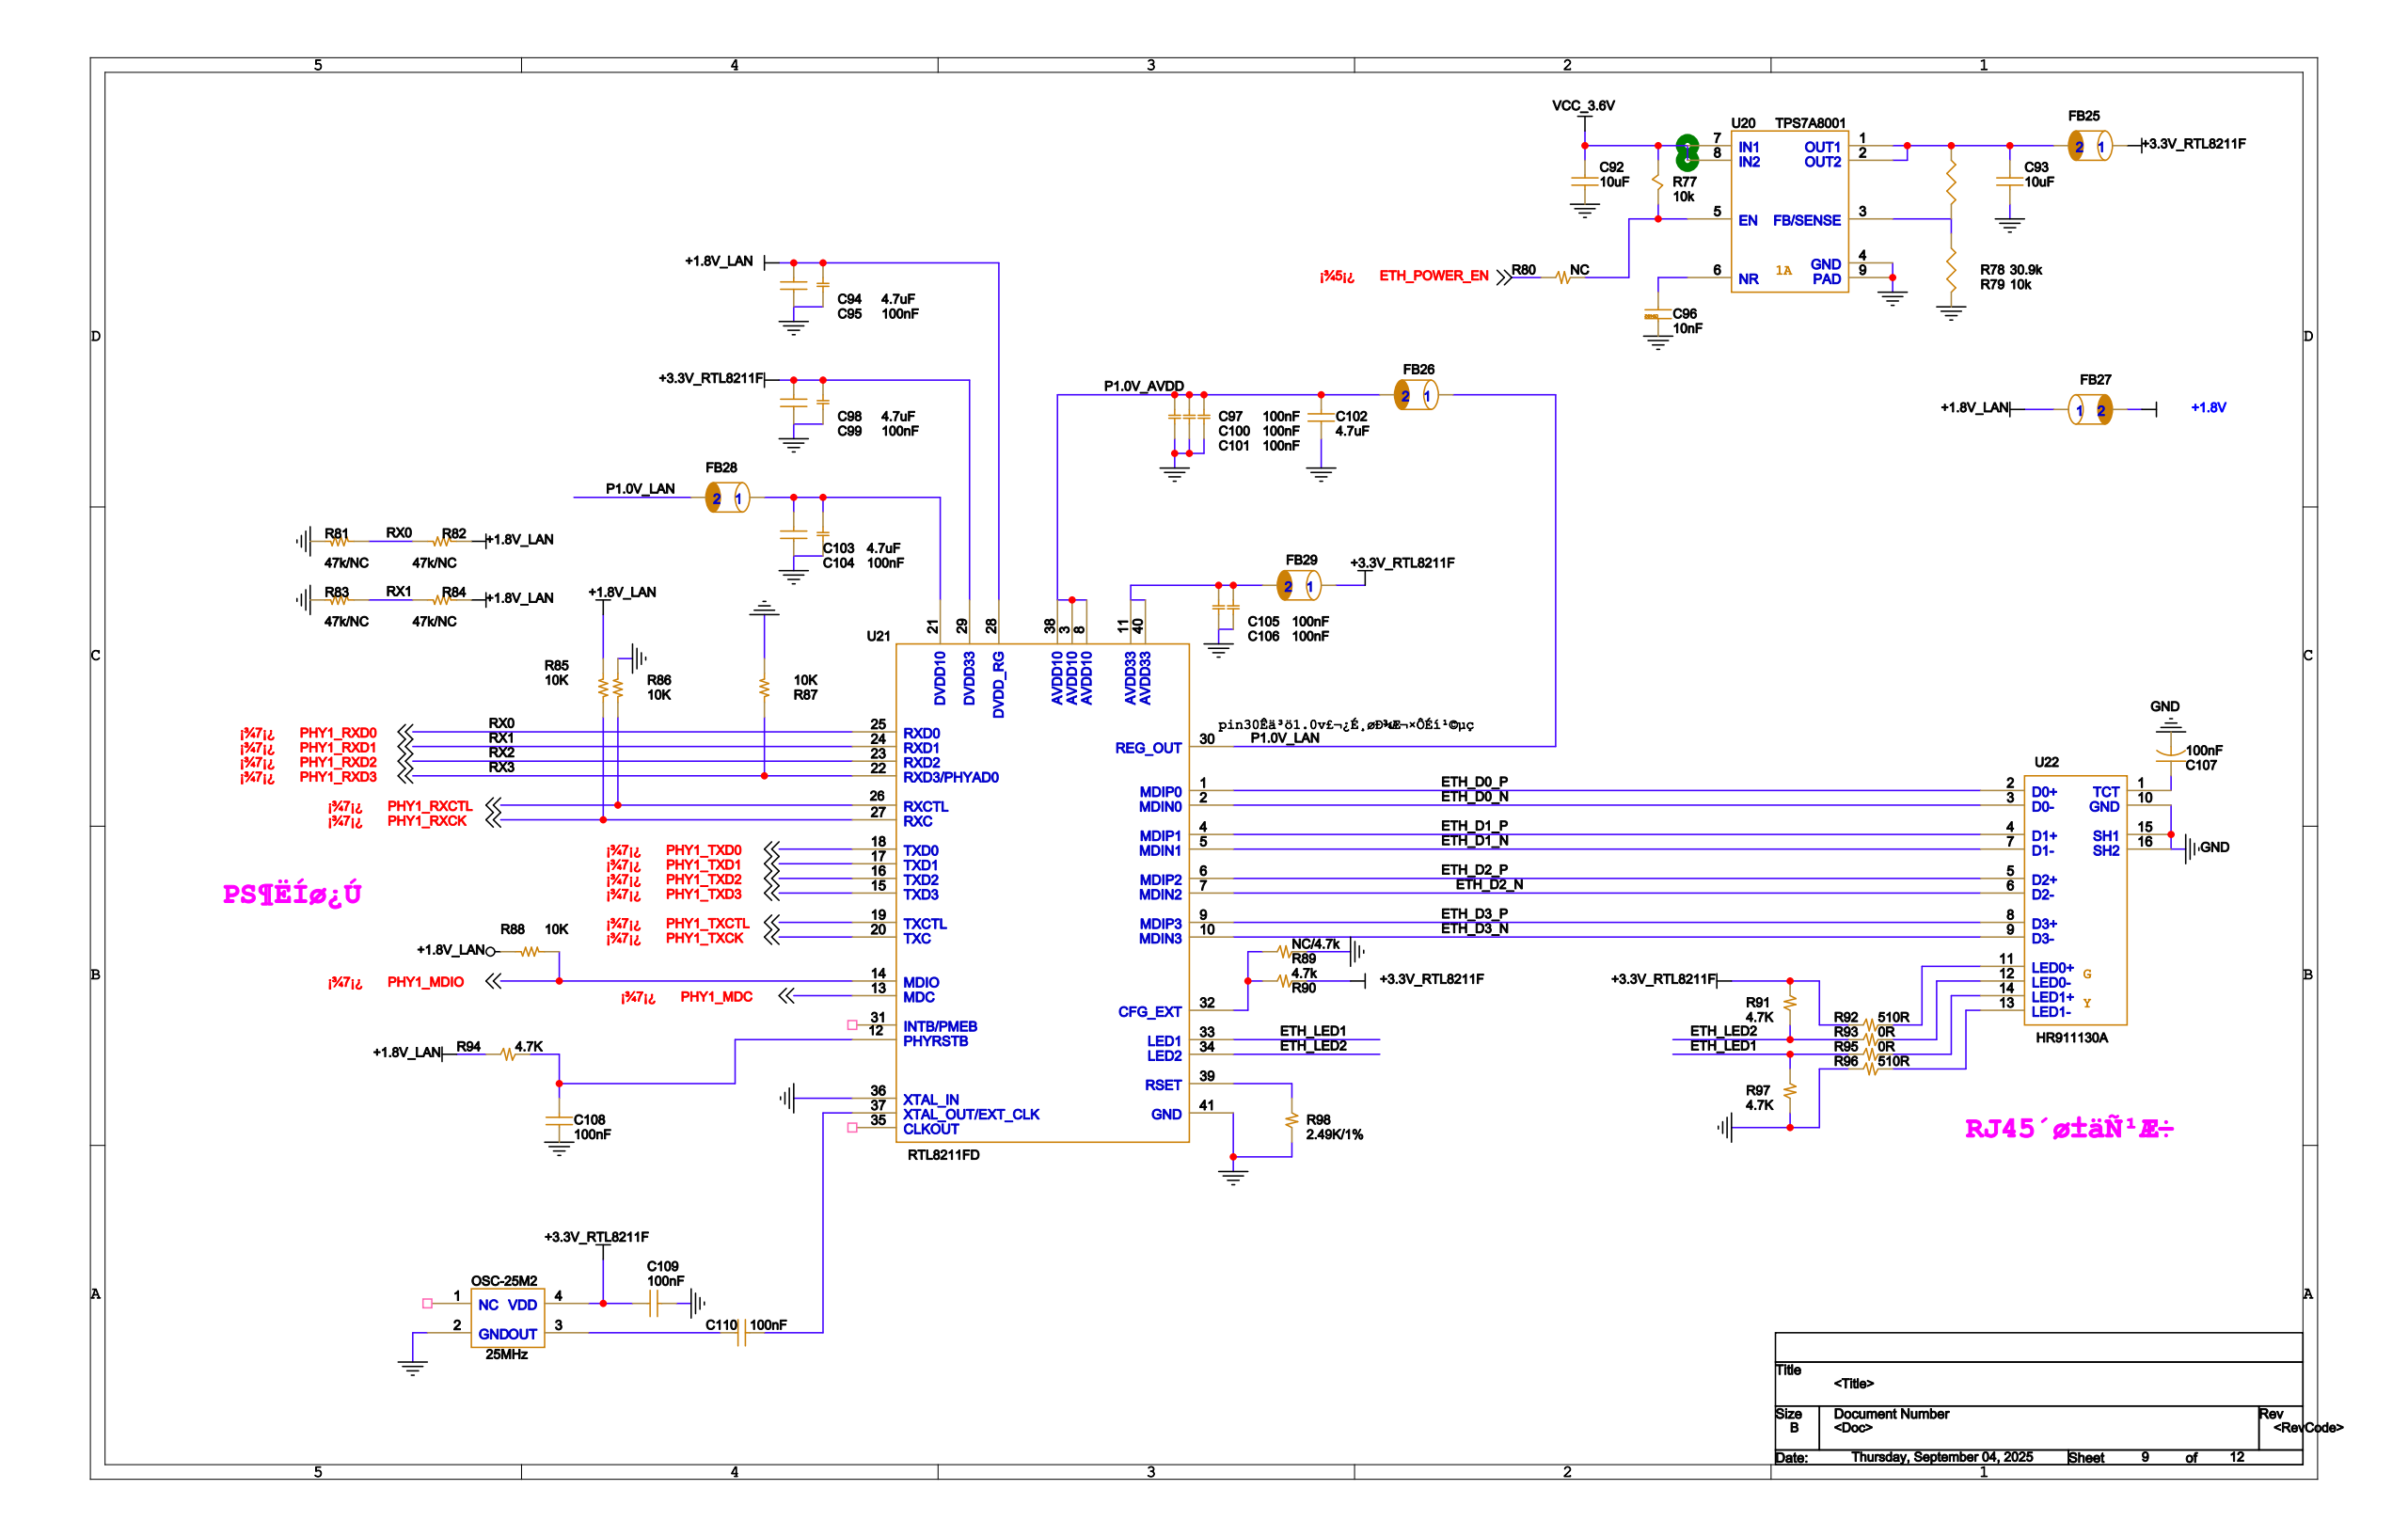Circuit board | Cadence Allegro | 528 parts | 530 nets | one sheet of the schematic
Parts on this sheet (reference | value | footprint):
C92 | 10uF | C0603
C93 | 10uF | C0603
C94 | 4.7uF | C0603
C95 | 100nF | C0402
C96 | 10nF | C0402
C97 | 100nF | C0402
C98 | 4.7uF | C0603
C99 | 100nF | C0402
C100 | 100nF | C0402
C101 | 100nF | C0402
C102 | 4.7uF | C0603
C103 | 4.7uF | C0603
C104 | 100nF | C0402
C105 | 100nF | C0402
C106 | 100nF | C0402
C107 | 100nF | C0402
C108 | 100nF | C0402
C109 | 100nF | C0402
C110 | 100nF | C0402
FB25 | BLM18PG121SN1 | 0603
FB26 | BLM18PG121SN1 | 0603
FB27 | BLM18PG121SN1 | 0603
FB28 | BLM18PG121SN1 | 0603
FB29 | BLM18PG121SN1 | 0603
OSC-25M2 | 25MHz | 3225-4
R77 | 10k | R0402
R78 | 30.9k | R0402
R79 | 10k | R0402
R80 | NC | R0402
R81 | 47k/NC | R0402
R82 | 47k/NC | R0402
R83 | 47k/NC | R0402
R84 | 47k/NC | R0402
R85 | 10K | R0402
R86 | 10K | R0402
R87 | 10K | R0402
R88 | 10K | R0402
R89 | NC/4.7k | R0402
R90 | 4.7k | R0402
R91 | 4.7k | R0402
R92 | 510R | R0402
R93 | 0R | R0402
R94 | 4.7k | R0402
R95 | 0R | R0402
R96 | 510R | R0402
R97 | 4.7k | R0402
R98 | 2.49K/1% | R0402
U20 | TPS7A8001 | TPS7A8001
U21 | RTL8211FD | RTL8211F
U22 | HR911130A | HR911130A
Nets of these parts (net: part-pin ...):
GND: C92-2 C93-2 C94-1 C95-2 C96-1 C97-2 C98-1 C99-2 C100-2 C101-2 C102-1 C103-1 C104-2 C105-2 C106-2 C107-2 C108-1 C109-2 OSC-25M2-2 R79-2 R81-2 R83-2 R86-2 R87-2 R89-1 R96-2 R97-2 R98-2 U20-4 U20-9 U22-10 U22-15 U22-16 U21-36 U21-41
VCC_3.6V: C92-1 R77-2 U20-7 U20-8
N18532011: R77-1 R80-2 U20-5
N18596062: R78-2 R79-1 U20-3
N18596078: C96-2 U20-6
N18596007: C93-1 FB25-2 R78-1 U20-1 U20-2
N19779312: C110-1 OSC-25M2-3
+3.3V_RTL8211F: C98-2 C99-1 C109-1 FB25-1 FB29-1 OSC-25M2-4 R90-1 R91-2 R92-2 U21-29
P1.0V_AVDD: C97-1 C100-1 C101-1 C102-2 FB26-2 U21-3 U21-8 U21-38
N19778543: C103-2 C104-1 FB28-1 U21-21
N19778594: C105-1 C106-1 FB29-2 U21-11 U21-40
+1.8V_LAN: C94-2 C95-1 FB27-1 R82-1 R84-1 R85-2 R88-2 R94-2 U21-28
N19801045: C107-1 U22-1
N18531892: C108-2 R94-1 U21-12
N19779246: C110-2 U21-37
+1.8V: FB27-2
P1.0V_LAN: FB26-1 FB28-2 U21-30
N19779036: R93-1 U22-12
ETH_LED2: R91-1 R93-2 U21-34
N19779057: R95-1 U22-14
ETH_LED1: R95-2 R97-1 U21-33
ETH_POWER_EN: R80-1
N18427484: R89-2 R90-2 U21-32
N19779023: R92-1 U22-11
N19779099: R96-1 U22-13
N19779234: R98-1 U21-39
PHY1_TXD0: U21-18
PHY1_TXCK: U21-20
PHY1_RXD1: R83-1 R84-2 U21-24
PHY1_TXD1: U21-17
PHY1_RXD2: U21-23
PHY1_TXCTL: U21-19
PHY1_RXD0: R81-1 R82-2 U21-25
PHY1_TXD2: U21-16
PHY1_RXD3: R87-1 U21-22
PHY1_MDIO: R88-1 U21-14
PHY1_RXCK: R85-1 U21-27
PHY1_MDC: U21-13
PHY1_TXD3: U21-15
PHY1_RXCTL: R86-1 U21-26
ETH_D0_N: U22-3 U21-2
ETH_D1_N: U22-7 U21-5
ETH_D2_N: U22-6 U21-7
ETH_D3_N: U22-9 U21-10
ETH_D0_P: U22-2 U21-1
ETH_D1_P: U22-4 U21-4
ETH_D2_P: U22-5 U21-6
ETH_D3_P: U22-8 U21-9